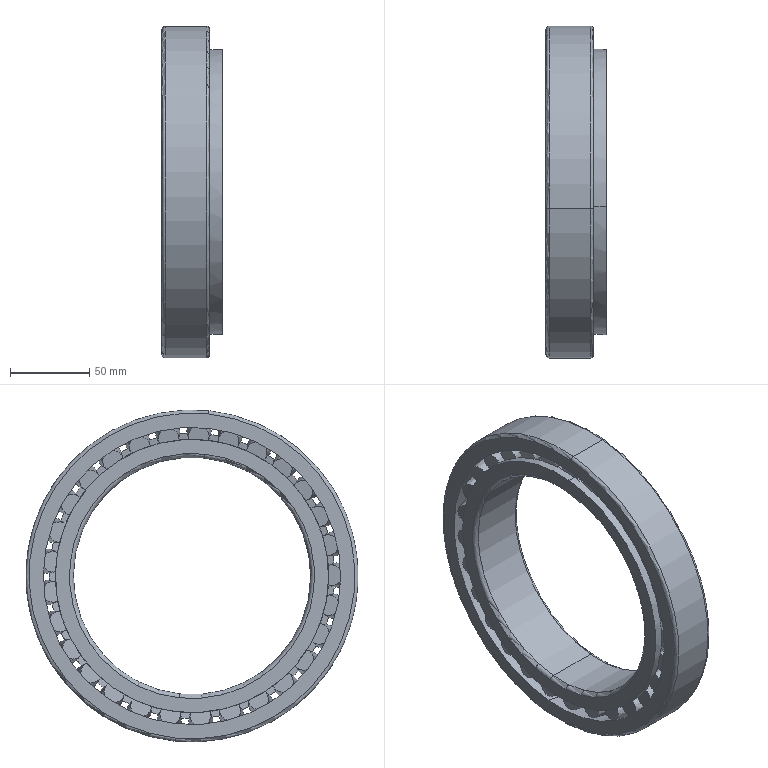Part | NX | features BREP 1 | 1 solid | 231 faces | box 38 x 210 x 210 mm | volume 453592 mm3 | cone 153 | plane 62 | torus 8 | cylinder 8 | commonest cylinder face diameters 150 x2 172.756 x2 180.341 x2 210 x2